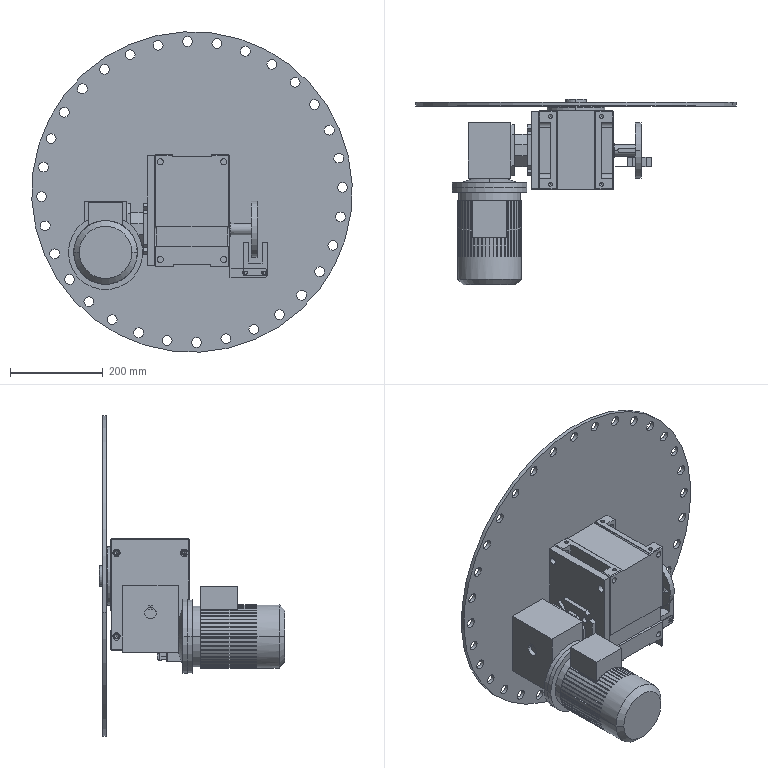Part | 10 solids | 994 faces | box 690 x 399 x 690 mm | volume 15196289 mm3 | plane 503 | cylinder 278 | spline 137 | cone 74 | torus 2 | commonest cylinder face diameters 21 x64 8.5 x34 8 x18 4.7 x16 13 x16 10 x13